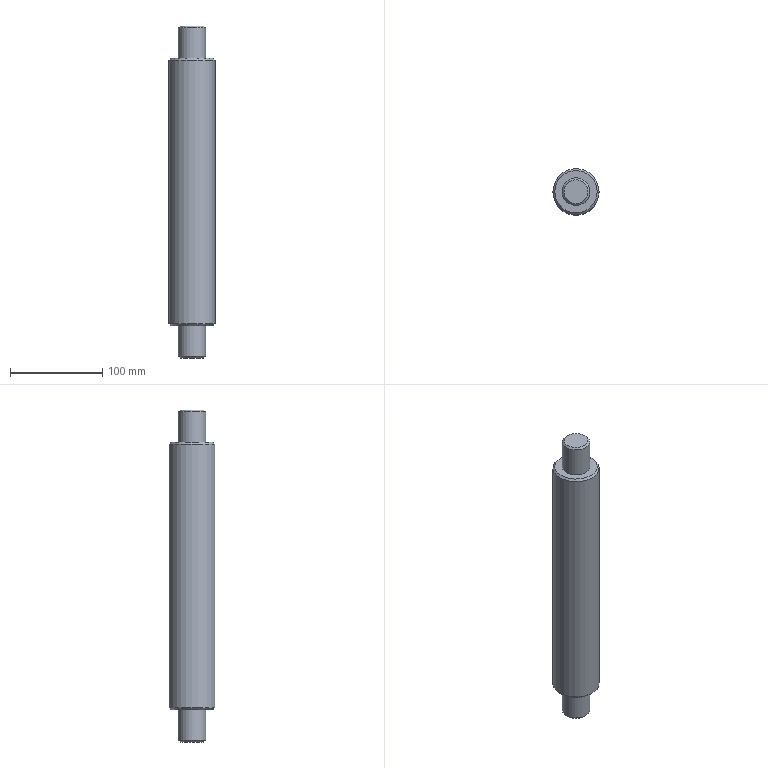Part | STEP file | solid 4 | 1 solid | 11 faces | box 50 x 50 x 360 mm | volume 617922 mm3 | plane 4 | cone 4 | cylinder 3 | commonest cylinder face diameters 30 x2 50 x1